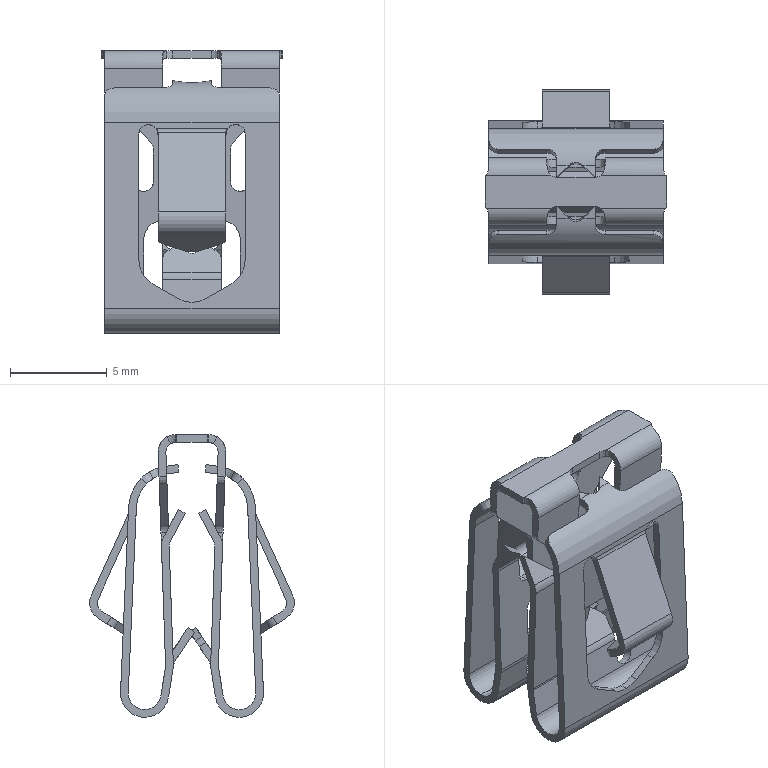Part | SolidWorks | features BaseBody 1 | 1 solid | 267 faces | box 9.4 x 10.589 x 14.619 mm | volume 169.677 mm3 | plane 123 | cylinder 116 | spline 28 | commonest cylinder face diameters 1 x72 1.8 x18 3 x8 2 x6 1.7 x3 2.5 x3